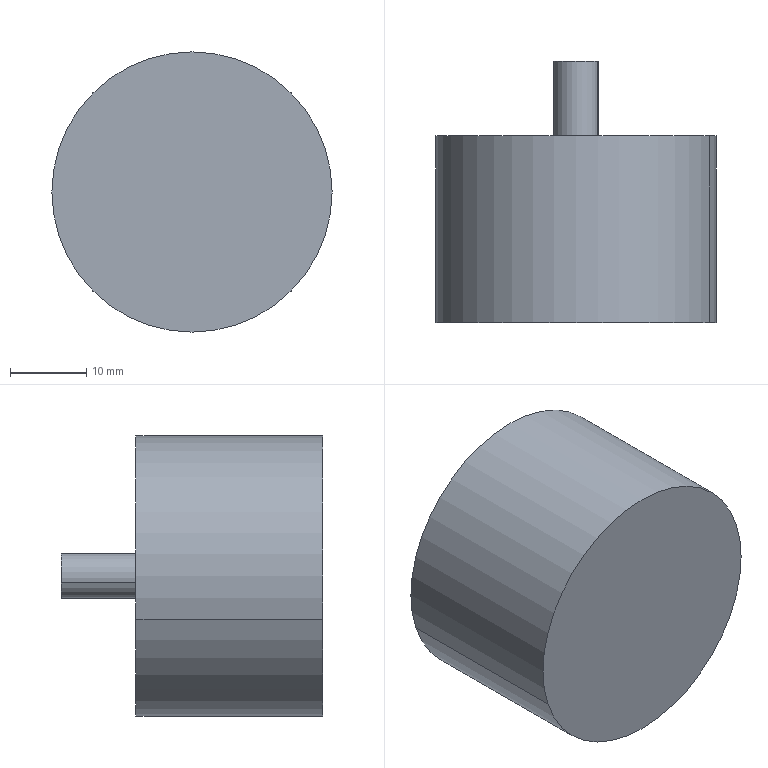Part | STEP file | 1 solid | 7 faces | box 36.75 x 34.3 x 36.75 mm | volume 26254 mm3 | cylinder 4 | plane 3 | commonest cylinder face diameters 5.88 x2 36.75 x2
STEP:
#1=CARTESIAN_POINT('',(0.,0.,0.));
#2=DIRECTION('',(0.,0.,1.));
#3=DIRECTION('',(1.,0.,0.));
#4=AXIS2_PLACEMENT_3D('',#1,#2,#3);
#5=CARTESIAN_POINT('',(848.214,-154.536,128.677));
#6=VERTEX_POINT('',#5);
#7=CARTESIAN_POINT('',(853.807,-154.536,130.494));
#8=VERTEX_POINT('',#7);
#9=CARTESIAN_POINT('',(851.01,-154.536,129.586));
#10=DIRECTION('',(0.,1.,0.));
#11=DIRECTION('',(0.9511,0.,0.309));
#12=AXIS2_PLACEMENT_3D('',#9,#10,#11);
#13=CIRCLE('',#12,2.94);
#14=CARTESIAN_POINT('',(851.01,-154.536,129.586));
#15=DIRECTION('',(0.,1.,0.));
#16=DIRECTION('',(0.309,0.,-0.9511));
#17=AXIS2_PLACEMENT_3D('',#14,#15,#16);
#18=PLANE('',#17);
#19=CARTESIAN_POINT('',(0.,0.));
#20=DIRECTION('',(0.,-1.));
#21=AXIS2_PLACEMENT_2D('',#19,#20);
#22=CIRCLE('',#21,2.94);
#23=(GEOMETRIC_REPRESENTATION_CONTEXT(2)PARAMETRIC_REPRESENTATION_CONTEXT()REPRESENTATION_CONTEXT('',''));
#24=DEFINITIONAL_REPRESENTATION('',(#22),#23);
#25=PCURVE('',#18,#24);
#26=CARTESIAN_POINT('',(851.01,-154.536,129.586));
#27=DIRECTION('',(0.,-1.,0.));
#28=DIRECTION('',(-0.9511,0.,-0.309));
#29=AXIS2_PLACEMENT_3D('',#26,#27,#28);
#30=CYLINDRICAL_SURFACE('',#29,2.94);
#31=CARTESIAN_POINT('',(9.425,0.));
#32=DIRECTION('',(-1.,0.));
#33=VECTOR('',#32,1.);
#34=LINE('',#31,#33);
#35=(GEOMETRIC_REPRESENTATION_CONTEXT(2)PARAMETRIC_REPRESENTATION_CONTEXT()REPRESENTATION_CONTEXT('',''));
#36=DEFINITIONAL_REPRESENTATION('',(#34),#35);
#37=PCURVE('',#30,#36);
#38=SURFACE_CURVE('',#13,(#25,#37),.PCURVE_S1.);
#39=EDGE_CURVE('',#6,#8,#38,.T.);
#40=ORIENTED_EDGE('',*,*,#39,.T.);
#41=CARTESIAN_POINT('',(851.01,-154.536,129.586));
#42=DIRECTION('',(0.,1.,0.));
#43=DIRECTION('',(0.9511,0.,0.309));
#44=AXIS2_PLACEMENT_3D('',#41,#42,#43);
#45=CIRCLE('',#44,2.94);
#46=CARTESIAN_POINT('',(0.,0.));
#47=DIRECTION('',(0.,-1.));
#48=AXIS2_PLACEMENT_2D('',#46,#47);
#49=CIRCLE('',#48,2.94);
#50=(GEOMETRIC_REPRESENTATION_CONTEXT(2)PARAMETRIC_REPRESENTATION_CONTEXT()REPRESENTATION_CONTEXT('',''));
#51=DEFINITIONAL_REPRESENTATION('',(#49),#50);
#52=PCURVE('',#18,#51);
#53=CARTESIAN_POINT('',(851.01,-154.536,129.586));
#54=DIRECTION('',(0.,-1.,0.));
#55=DIRECTION('',(-0.9511,0.,-0.309));
#56=AXIS2_PLACEMENT_3D('',#53,#54,#55);
#57=CYLINDRICAL_SURFACE('',#56,2.94);
#58=CARTESIAN_POINT('',(3.142,0.));
#59=DIRECTION('',(-1.,0.));
#60=VECTOR('',#59,1.);
#61=LINE('',#58,#60);
#62=(GEOMETRIC_REPRESENTATION_CONTEXT(2)PARAMETRIC_REPRESENTATION_CONTEXT()REPRESENTATION_CONTEXT('',''));
#63=DEFINITIONAL_REPRESENTATION('',(#61),#62);
#64=PCURVE('',#57,#63);
#65=SURFACE_CURVE('',#45,(#52,#64),.PCURVE_S1.);
#66=EDGE_CURVE('',#8,#6,#65,.T.);
#67=ORIENTED_EDGE('',*,*,#66,.T.);
#68=EDGE_LOOP('',(#40,#67));
#69=FACE_BOUND('',#68,.T.);
#70=ADVANCED_FACE('',(#69),#18,.T.);
#71=CARTESIAN_POINT('',(853.807,-164.336,130.494));
#72=VERTEX_POINT('',#71);
#73=CARTESIAN_POINT('',(853.807,-154.536,130.494));
#74=DIRECTION('',(0.,-1.,0.));
#75=VECTOR('',#74,1.);
#76=LINE('',#73,#75);
#77=CARTESIAN_POINT('',(3.142,0.));
#78=DIRECTION('',(0.,1.));
#79=VECTOR('',#78,1.);
#80=LINE('',#77,#79);
#81=(GEOMETRIC_REPRESENTATION_CONTEXT(2)PARAMETRIC_REPRESENTATION_CONTEXT()REPRESENTATION_CONTEXT('',''));
#82=DEFINITIONAL_REPRESENTATION('',(#80),#81);
#83=PCURVE('',#30,#82);
#84=CARTESIAN_POINT('',(3.142,0.));
#85=DIRECTION('',(0.,1.));
#86=VECTOR('',#85,1.);
#87=LINE('',#84,#86);
#88=(GEOMETRIC_REPRESENTATION_CONTEXT(2)PARAMETRIC_REPRESENTATION_CONTEXT()REPRESENTATION_CONTEXT('',''));
#89=DEFINITIONAL_REPRESENTATION('',(#87),#88);
#90=PCURVE('',#57,#89);
#91=SURFACE_CURVE('',#76,(#83,#90),.PCURVE_S1.);
#92=EDGE_CURVE('',#8,#72,#91,.T.);
#93=ORIENTED_EDGE('',*,*,#92,.F.);
#94=ORIENTED_EDGE('',*,*,#39,.F.);
#95=CARTESIAN_POINT('',(848.214,-164.336,128.677));
#96=VERTEX_POINT('',#95);
#97=CARTESIAN_POINT('',(848.214,-154.536,128.677));
#98=DIRECTION('',(0.,-1.,0.));
#99=VECTOR('',#98,1.);
#100=LINE('',#97,#99);
#101=CARTESIAN_POINT('',(6.283,0.));
#102=DIRECTION('',(0.,1.));
#103=VECTOR('',#102,1.);
#104=LINE('',#101,#103);
#105=(GEOMETRIC_REPRESENTATION_CONTEXT(2)PARAMETRIC_REPRESENTATION_CONTEXT()REPRESENTATION_CONTEXT('',''));
#106=DEFINITIONAL_REPRESENTATION('',(#104),#105);
#107=PCURVE('',#30,#106);
#108=CARTESIAN_POINT('',(0.,0.));
#109=DIRECTION('',(0.,1.));
#110=VECTOR('',#109,1.);
#111=LINE('',#108,#110);
#112=(GEOMETRIC_REPRESENTATION_CONTEXT(2)PARAMETRIC_REPRESENTATION_CONTEXT()REPRESENTATION_CONTEXT('',''));
#113=DEFINITIONAL_REPRESENTATION('',(#111),#112);
#114=PCURVE('',#57,#113);
#115=SURFACE_CURVE('',#100,(#107,#114),.PCURVE_S1.);
#116=EDGE_CURVE('',#6,#96,#115,.T.);
#117=ORIENTED_EDGE('',*,*,#116,.T.);
#118=CARTESIAN_POINT('',(851.01,-164.336,129.586));
#119=DIRECTION('',(0.,1.,0.));
#120=DIRECTION('',(0.9511,0.,0.309));
#121=AXIS2_PLACEMENT_3D('',#118,#119,#120);
#122=CIRCLE('',#121,2.94);
#123=CARTESIAN_POINT('',(9.425,9.8));
#124=DIRECTION('',(-1.,0.));
#125=VECTOR('',#124,1.);
#126=LINE('',#123,#125);
#127=(GEOMETRIC_REPRESENTATION_CONTEXT(2)PARAMETRIC_REPRESENTATION_CONTEXT()REPRESENTATION_CONTEXT('',''));
#128=DEFINITIONAL_REPRESENTATION('',(#126),#127);
#129=PCURVE('',#30,#128);
#130=CARTESIAN_POINT('',(851.01,-164.336,129.586));
#131=DIRECTION('',(0.,1.,0.));
#132=DIRECTION('',(0.309,0.,-0.9511));
#133=AXIS2_PLACEMENT_3D('',#130,#131,#132);
#134=PLANE('',#133);
#135=CARTESIAN_POINT('',(0.,0.));
#136=DIRECTION('',(0.,-1.));
#137=AXIS2_PLACEMENT_2D('',#135,#136);
#138=CIRCLE('',#137,2.94);
#139=(GEOMETRIC_REPRESENTATION_CONTEXT(2)PARAMETRIC_REPRESENTATION_CONTEXT()REPRESENTATION_CONTEXT('',''));
#140=DEFINITIONAL_REPRESENTATION('',(#138),#139);
#141=PCURVE('',#134,#140);
#142=SURFACE_CURVE('',#122,(#129,#141),.PCURVE_S1.);
#143=EDGE_CURVE('',#96,#72,#142,.T.);
#144=ORIENTED_EDGE('',*,*,#143,.T.);
#145=EDGE_LOOP('',(#93,#94,#117,#144));
#146=FACE_BOUND('',#145,.T.);
#147=ADVANCED_FACE('',(#146),#30,.T.);
#148=CARTESIAN_POINT('',(833.535,-188.836,123.907));
#149=VERTEX_POINT('',#148);
#150=CARTESIAN_POINT('',(868.486,-188.836,135.264));
#151=VERTEX_POINT('',#150);
#152=CARTESIAN_POINT('',(851.01,-188.836,129.586));
#153=DIRECTION('',(0.,1.,0.));
#154=DIRECTION('',(0.9511,0.,0.309));
#155=AXIS2_PLACEMENT_3D('',#152,#153,#154);
#156=CIRCLE('',#155,18.375);
#157=CARTESIAN_POINT('',(851.01,-188.836,129.586));
#158=DIRECTION('',(0.,1.,0.));
#159=DIRECTION('',(0.309,0.,-0.9511));
#160=AXIS2_PLACEMENT_3D('',#157,#158,#159);
#161=PLANE('',#160);
#162=CARTESIAN_POINT('',(0.,0.));
#163=DIRECTION('',(0.,-1.));
#164=AXIS2_PLACEMENT_2D('',#162,#163);
#165=CIRCLE('',#164,18.375);
#166=(GEOMETRIC_REPRESENTATION_CONTEXT(2)PARAMETRIC_REPRESENTATION_CONTEXT()REPRESENTATION_CONTEXT('',''));
#167=DEFINITIONAL_REPRESENTATION('',(#165),#166);
#168=PCURVE('',#161,#167);
#169=CARTESIAN_POINT('',(851.01,-164.336,129.586));
#170=DIRECTION('',(0.,-1.,0.));
#171=DIRECTION('',(-0.9511,0.,-0.309));
#172=AXIS2_PLACEMENT_3D('',#169,#170,#171);
#173=CYLINDRICAL_SURFACE('',#172,18.375);
#174=CARTESIAN_POINT('',(9.425,24.5));
#175=DIRECTION('',(-1.,0.));
#176=VECTOR('',#175,1.);
#177=LINE('',#174,#176);
#178=(GEOMETRIC_REPRESENTATION_CONTEXT(2)PARAMETRIC_REPRESENTATION_CONTEXT()REPRESENTATION_CONTEXT('',''));
#179=DEFINITIONAL_REPRESENTATION('',(#177),#178);
#180=PCURVE('',#173,#179);
#181=SURFACE_CURVE('',#156,(#168,#180),.PCURVE_S1.);
#182=EDGE_CURVE('',#149,#151,#181,.T.);
#183=ORIENTED_EDGE('',*,*,#182,.F.);
#184=CARTESIAN_POINT('',(851.01,-188.836,129.586));
#185=DIRECTION('',(0.,1.,0.));
#186=DIRECTION('',(0.9511,0.,0.309));
#187=AXIS2_PLACEMENT_3D('',#184,#185,#186);
#188=CIRCLE('',#187,18.375);
#189=CARTESIAN_POINT('',(0.,0.));
#190=DIRECTION('',(0.,-1.));
#191=AXIS2_PLACEMENT_2D('',#189,#190);
#192=CIRCLE('',#191,18.375);
#193=(GEOMETRIC_REPRESENTATION_CONTEXT(2)PARAMETRIC_REPRESENTATION_CONTEXT()REPRESENTATION_CONTEXT('',''));
#194=DEFINITIONAL_REPRESENTATION('',(#192),#193);
#195=PCURVE('',#161,#194);
#196=CARTESIAN_POINT('',(851.01,-164.336,129.586));
#197=DIRECTION('',(0.,-1.,0.));
#198=DIRECTION('',(-0.9511,0.,-0.309));
#199=AXIS2_PLACEMENT_3D('',#196,#197,#198);
#200=CYLINDRICAL_SURFACE('',#199,18.375);
#201=CARTESIAN_POINT('',(3.142,24.5));
#202=DIRECTION('',(-1.,0.));
#203=VECTOR('',#202,1.);
#204=LINE('',#201,#203);
#205=(GEOMETRIC_REPRESENTATION_CONTEXT(2)PARAMETRIC_REPRESENTATION_CONTEXT()REPRESENTATION_CONTEXT('',''));
#206=DEFINITIONAL_REPRESENTATION('',(#204),#205);
#207=PCURVE('',#200,#206);
#208=SURFACE_CURVE('',#188,(#195,#207),.PCURVE_S1.);
#209=EDGE_CURVE('',#151,#149,#208,.T.);
#210=ORIENTED_EDGE('',*,*,#209,.F.);
#211=EDGE_LOOP('',(#183,#210));
#212=FACE_BOUND('',#211,.T.);
#213=ADVANCED_FACE('',(#212),#161,.F.);
#214=ORIENTED_EDGE('',*,*,#143,.F.);
#215=CARTESIAN_POINT('',(851.01,-164.336,129.586));
#216=DIRECTION('',(0.,1.,0.));
#217=DIRECTION('',(0.9511,0.,0.309));
#218=AXIS2_PLACEMENT_3D('',#215,#216,#217);
#219=CIRCLE('',#218,2.94);
#220=CARTESIAN_POINT('',(0.,0.));
#221=DIRECTION('',(0.,-1.));
#222=AXIS2_PLACEMENT_2D('',#220,#221);
#223=CIRCLE('',#222,2.94);
#224=(GEOMETRIC_REPRESENTATION_CONTEXT(2)PARAMETRIC_REPRESENTATION_CONTEXT()REPRESENTATION_CONTEXT('',''));
#225=DEFINITIONAL_REPRESENTATION('',(#223),#224);
#226=PCURVE('',#134,#225);
#227=CARTESIAN_POINT('',(3.142,9.8));
#228=DIRECTION('',(-1.,0.));
#229=VECTOR('',#228,1.);
#230=LINE('',#227,#229);
#231=(GEOMETRIC_REPRESENTATION_CONTEXT(2)PARAMETRIC_REPRESENTATION_CONTEXT()REPRESENTATION_CONTEXT('',''));
#232=DEFINITIONAL_REPRESENTATION('',(#230),#231);
#233=PCURVE('',#57,#232);
#234=SURFACE_CURVE('',#219,(#226,#233),.PCURVE_S1.);
#235=EDGE_CURVE('',#72,#96,#234,.T.);
#236=ORIENTED_EDGE('',*,*,#235,.F.);
#237=EDGE_LOOP('',(#214,#236));
#238=FACE_BOUND('',#237,.T.);
#239=CARTESIAN_POINT('',(833.535,-164.336,123.907));
#240=VERTEX_POINT('',#239);
#241=CARTESIAN_POINT('',(868.486,-164.336,135.264));
#242=VERTEX_POINT('',#241);
#243=CARTESIAN_POINT('',(851.01,-164.336,129.586));
#244=DIRECTION('',(0.,1.,0.));
#245=DIRECTION('',(0.9511,0.,0.309));
#246=AXIS2_PLACEMENT_3D('',#243,#244,#245);
#247=CIRCLE('',#246,18.375);
#248=CARTESIAN_POINT('',(0.,0.));
#249=DIRECTION('',(0.,-1.));
#250=AXIS2_PLACEMENT_2D('',#248,#249);
#251=CIRCLE('',#250,18.375);
#252=(GEOMETRIC_REPRESENTATION_CONTEXT(2)PARAMETRIC_REPRESENTATION_CONTEXT()REPRESENTATION_CONTEXT('',''));
#253=DEFINITIONAL_REPRESENTATION('',(#251),#252);
#254=PCURVE('',#134,#253);
#255=CARTESIAN_POINT('',(9.425,0.));
#256=DIRECTION('',(-1.,0.));
#257=VECTOR('',#256,1.);
#258=LINE('',#255,#257);
#259=(GEOMETRIC_REPRESENTATION_CONTEXT(2)PARAMETRIC_REPRESENTATION_CONTEXT()REPRESENTATION_CONTEXT('',''));
#260=DEFINITIONAL_REPRESENTATION('',(#258),#259);
#261=PCURVE('',#173,#260);
#262=SURFACE_CURVE('',#247,(#254,#261),.PCURVE_S1.);
#263=EDGE_CURVE('',#240,#242,#262,.T.);
#264=ORIENTED_EDGE('',*,*,#263,.T.);
#265=CARTESIAN_POINT('',(851.01,-164.336,129.586));
#266=DIRECTION('',(0.,1.,0.));
#267=DIRECTION('',(0.9511,0.,0.309));
#268=AXIS2_PLACEMENT_3D('',#265,#266,#267);
#269=CIRCLE('',#268,18.375);
#270=CARTESIAN_POINT('',(0.,0.));
#271=DIRECTION('',(0.,-1.));
#272=AXIS2_PLACEMENT_2D('',#270,#271);
#273=CIRCLE('',#272,18.375);
#274=(GEOMETRIC_REPRESENTATION_CONTEXT(2)PARAMETRIC_REPRESENTATION_CONTEXT()REPRESENTATION_CONTEXT('',''));
#275=DEFINITIONAL_REPRESENTATION('',(#273),#274);
#276=PCURVE('',#134,#275);
#277=CARTESIAN_POINT('',(3.142,0.));
#278=DIRECTION('',(-1.,0.));
#279=VECTOR('',#278,1.);
#280=LINE('',#277,#279);
#281=(GEOMETRIC_REPRESENTATION_CONTEXT(2)PARAMETRIC_REPRESENTATION_CONTEXT()REPRESENTATION_CONTEXT('',''));
#282=DEFINITIONAL_REPRESENTATION('',(#280),#281);
#283=PCURVE('',#200,#282);
#284=SURFACE_CURVE('',#269,(#276,#283),.PCURVE_S1.);
#285=EDGE_CURVE('',#242,#240,#284,.T.);
#286=ORIENTED_EDGE('',*,*,#285,.T.);
#287=EDGE_LOOP('',(#264,#286));
#288=FACE_BOUND('',#287,.T.);
#289=ADVANCED_FACE('',(#238,#288),#134,.T.);
#290=CARTESIAN_POINT('',(868.486,-164.336,135.264));
#291=DIRECTION('',(0.,-1.,0.));
#292=VECTOR('',#291,1.);
#293=LINE('',#290,#292);
#294=CARTESIAN_POINT('',(3.142,0.));
#295=DIRECTION('',(0.,1.));
#296=VECTOR('',#295,1.);
#297=LINE('',#294,#296);
#298=(GEOMETRIC_REPRESENTATION_CONTEXT(2)PARAMETRIC_REPRESENTATION_CONTEXT()REPRESENTATION_CONTEXT('',''));
#299=DEFINITIONAL_REPRESENTATION('',(#297),#298);
#300=PCURVE('',#173,#299);
#301=CARTESIAN_POINT('',(3.142,0.));
#302=DIRECTION('',(0.,1.));
#303=VECTOR('',#302,1.);
#304=LINE('',#301,#303);
#305=(GEOMETRIC_REPRESENTATION_CONTEXT(2)PARAMETRIC_REPRESENTATION_CONTEXT()REPRESENTATION_CONTEXT('',''));
#306=DEFINITIONAL_REPRESENTATION('',(#304),#305);
#307=PCURVE('',#200,#306);
#308=SURFACE_CURVE('',#293,(#300,#307),.PCURVE_S1.);
#309=EDGE_CURVE('',#242,#151,#308,.T.);
#310=ORIENTED_EDGE('',*,*,#309,.F.);
#311=ORIENTED_EDGE('',*,*,#263,.F.);
#312=CARTESIAN_POINT('',(833.535,-164.336,123.907));
#313=DIRECTION('',(0.,-1.,0.));
#314=VECTOR('',#313,1.);
#315=LINE('',#312,#314);
#316=CARTESIAN_POINT('',(6.283,0.));
#317=DIRECTION('',(0.,1.));
#318=VECTOR('',#317,1.);
#319=LINE('',#316,#318);
#320=(GEOMETRIC_REPRESENTATION_CONTEXT(2)PARAMETRIC_REPRESENTATION_CONTEXT()REPRESENTATION_CONTEXT('',''));
#321=DEFINITIONAL_REPRESENTATION('',(#319),#320);
#322=PCURVE('',#173,#321);
#323=CARTESIAN_POINT('',(0.,0.));
#324=DIRECTION('',(0.,1.));
#325=VECTOR('',#324,1.);
#326=LINE('',#323,#325);
#327=(GEOMETRIC_REPRESENTATION_CONTEXT(2)PARAMETRIC_REPRESENTATION_CONTEXT()REPRESENTATION_CONTEXT('',''));
#328=DEFINITIONAL_REPRESENTATION('',(#326),#327);
#329=PCURVE('',#200,#328);
#330=SURFACE_CURVE('',#315,(#322,#329),.PCURVE_S1.);
#331=EDGE_CURVE('',#240,#149,#330,.T.);
#332=ORIENTED_EDGE('',*,*,#331,.T.);
#333=ORIENTED_EDGE('',*,*,#182,.T.);
#334=EDGE_LOOP('',(#310,#311,#332,#333));
#335=FACE_BOUND('',#334,.T.);
#336=ADVANCED_FACE('',(#335),#173,.T.);
#337=ORIENTED_EDGE('',*,*,#285,.F.);
#338=ORIENTED_EDGE('',*,*,#309,.T.);
#339=ORIENTED_EDGE('',*,*,#209,.T.);
#340=ORIENTED_EDGE('',*,*,#331,.F.);
#341=EDGE_LOOP('',(#337,#338,#339,#340));
#342=FACE_BOUND('',#341,.T.);
#343=ADVANCED_FACE('',(#342),#200,.T.);
#344=ORIENTED_EDGE('',*,*,#66,.F.);
#345=ORIENTED_EDGE('',*,*,#92,.T.);
#346=ORIENTED_EDGE('',*,*,#235,.T.);
#347=ORIENTED_EDGE('',*,*,#116,.F.);
#348=EDGE_LOOP('',(#344,#345,#346,#347));
#349=FACE_BOUND('',#348,.T.);
#350=ADVANCED_FACE('',(#349),#57,.T.);
#351=CLOSED_SHELL('',(#70,#147,#213,#289,#336,#343,#350));
#352=MANIFOLD_SOLID_BREP('',#351);
#353=(LENGTH_UNIT()NAMED_UNIT(*)SI_UNIT(.MILLI.,.METRE.));
#354=UNCERTAINTY_MEASURE_WITH_UNIT(LENGTH_MEASURE(0.0000001),#353,'','');
#355=(NAMED_UNIT(*)PLANE_ANGLE_UNIT()SI_UNIT($,.RADIAN.));
#356=(NAMED_UNIT(*)SI_UNIT($,.STERADIAN.)SOLID_ANGLE_UNIT());
#357=(GEOMETRIC_REPRESENTATION_CONTEXT(3)GLOBAL_UNCERTAINTY_ASSIGNED_CONTEXT((#354))GLOBAL_UNIT_ASSIGNED_CONTEXT((#353,#355,#356))REPRESENTATION_CONTEXT('',''));
#358=ADVANCED_BREP_SHAPE_REPRESENTATION('',(#4,#352),#357);